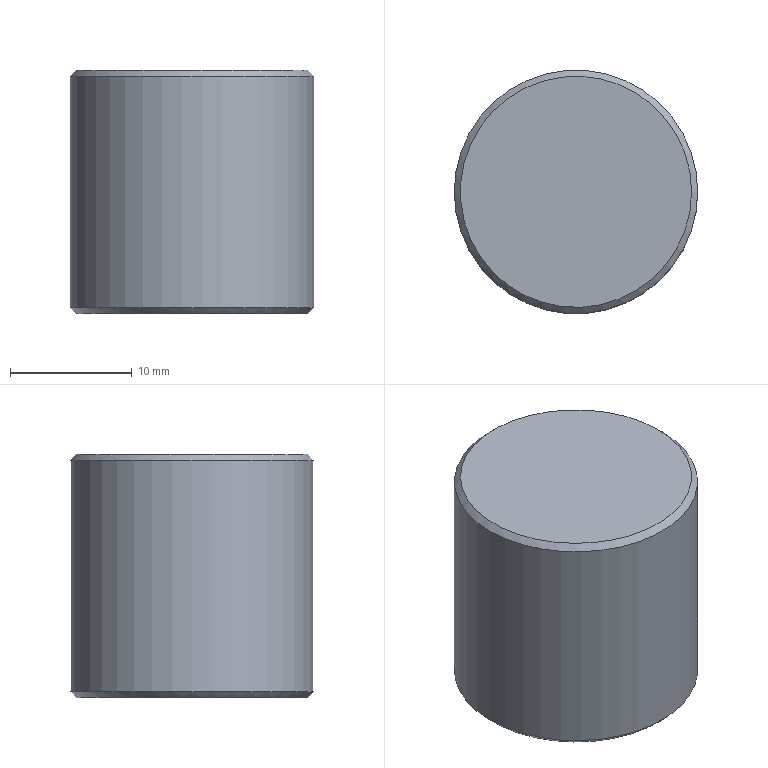Part | STEP file | E112002500 | 1 solid | 5 faces | box 20 x 20 x 20 mm | volume 6268 mm3 | plane 2 | cone 2 | cylinder 1 | commonest cylinder face diameters 20 x1
STEP:
#1=CARTESIAN_POINT('',(0.,0.,0.));
#2=DIRECTION('',(0.,0.,1.));
#3=DIRECTION('',(1.,0.,0.));
#4=AXIS2_PLACEMENT_3D('',#1,#2,#3);
#5=CARTESIAN_POINT('',(10.,0.,-0.5));
#6=VERTEX_POINT('',#5);
#7=CARTESIAN_POINT('',(0.,0.,-0.5));
#8=DIRECTION('',(0.,0.,-1.));
#9=DIRECTION('',(1.,0.,0.));
#10=AXIS2_PLACEMENT_3D('',#7,#8,#9);
#11=CIRCLE('',#10,10.);
#12=CARTESIAN_POINT('',(0.,0.,-20.));
#13=DIRECTION('',(0.,0.,1.));
#14=DIRECTION('',(1.,0.,0.));
#15=AXIS2_PLACEMENT_3D('',#12,#13,#14);
#16=CYLINDRICAL_SURFACE('',#15,10.);
#17=CARTESIAN_POINT('',(6.283,19.5));
#18=DIRECTION('',(-1.,0.));
#19=VECTOR('',#18,1.);
#20=LINE('',#17,#19);
#21=(GEOMETRIC_REPRESENTATION_CONTEXT(2)PARAMETRIC_REPRESENTATION_CONTEXT()REPRESENTATION_CONTEXT('',''));
#22=DEFINITIONAL_REPRESENTATION('',(#20),#21);
#23=PCURVE('',#16,#22);
#24=CARTESIAN_POINT('',(0.,0.,0.));
#25=DIRECTION('',(0.,0.,-1.));
#26=DIRECTION('',(-1.,0.,0.));
#27=AXIS2_PLACEMENT_3D('',#24,#25,#26);
#28=CONICAL_SURFACE('',#27,9.5,0.7854);
#29=CARTESIAN_POINT('',(3.142,0.5));
#30=DIRECTION('',(1.,0.));
#31=VECTOR('',#30,1.);
#32=LINE('',#29,#31);
#33=(GEOMETRIC_REPRESENTATION_CONTEXT(2)PARAMETRIC_REPRESENTATION_CONTEXT()REPRESENTATION_CONTEXT('',''));
#34=DEFINITIONAL_REPRESENTATION('',(#32),#33);
#35=PCURVE('',#28,#34);
#36=SURFACE_CURVE('',#11,(#23,#35),.PCURVE_S1.);
#37=EDGE_CURVE('',#6,#6,#36,.T.);
#38=ORIENTED_EDGE('',*,*,#37,.T.);
#39=CARTESIAN_POINT('',(10.,0.,-19.5));
#40=VERTEX_POINT('',#39);
#41=CARTESIAN_POINT('',(10.,0.,-19.5));
#42=CARTESIAN_POINT('',(10.,0.,-0.5));
#43=B_SPLINE_CURVE_WITH_KNOTS('',1,(#41,#42),.UNSPECIFIED.,.F.,.F.,(2,2),(0.5,19.5),.PIECEWISE_BEZIER_KNOTS.);
#44=CARTESIAN_POINT('',(0.,0.));
#45=DIRECTION('',(0.,1.));
#46=VECTOR('',#45,1.);
#47=LINE('',#44,#46);
#48=(GEOMETRIC_REPRESENTATION_CONTEXT(2)PARAMETRIC_REPRESENTATION_CONTEXT()REPRESENTATION_CONTEXT('',''));
#49=DEFINITIONAL_REPRESENTATION('',(#47),#48);
#50=PCURVE('',#16,#49);
#51=CARTESIAN_POINT('',(6.283,0.));
#52=DIRECTION('',(0.,1.));
#53=VECTOR('',#52,1.);
#54=LINE('',#51,#53);
#55=(GEOMETRIC_REPRESENTATION_CONTEXT(2)PARAMETRIC_REPRESENTATION_CONTEXT()REPRESENTATION_CONTEXT('',''));
#56=DEFINITIONAL_REPRESENTATION('',(#54),#55);
#57=PCURVE('',#16,#56);
#58=SEAM_CURVE('',#43,(#50,#57),.PCURVE_S1.);
#59=EDGE_CURVE('',#40,#6,#58,.T.);
#60=ORIENTED_EDGE('',*,*,#59,.F.);
#61=CARTESIAN_POINT('',(0.,0.,-19.5));
#62=DIRECTION('',(0.,0.,1.));
#63=DIRECTION('',(1.,0.,0.));
#64=AXIS2_PLACEMENT_3D('',#61,#62,#63);
#65=CIRCLE('',#64,10.);
#66=CARTESIAN_POINT('',(0.,0.5));
#67=DIRECTION('',(1.,0.));
#68=VECTOR('',#67,1.);
#69=LINE('',#66,#68);
#70=(GEOMETRIC_REPRESENTATION_CONTEXT(2)PARAMETRIC_REPRESENTATION_CONTEXT()REPRESENTATION_CONTEXT('',''));
#71=DEFINITIONAL_REPRESENTATION('',(#69),#70);
#72=PCURVE('',#16,#71);
#73=CARTESIAN_POINT('',(0.,0.,-19.5));
#74=DIRECTION('',(0.,0.,1.));
#75=DIRECTION('',(1.,0.,0.));
#76=AXIS2_PLACEMENT_3D('',#73,#74,#75);
#77=CONICAL_SURFACE('',#76,10.,0.7854);
#78=CARTESIAN_POINT('',(0.,0.));
#79=DIRECTION('',(1.,0.));
#80=VECTOR('',#79,1.);
#81=LINE('',#78,#80);
#82=(GEOMETRIC_REPRESENTATION_CONTEXT(2)PARAMETRIC_REPRESENTATION_CONTEXT()REPRESENTATION_CONTEXT('',''));
#83=DEFINITIONAL_REPRESENTATION('',(#81),#82);
#84=PCURVE('',#77,#83);
#85=SURFACE_CURVE('',#65,(#72,#84),.PCURVE_S1.);
#86=EDGE_CURVE('',#40,#40,#85,.T.);
#87=ORIENTED_EDGE('',*,*,#86,.T.);
#88=ORIENTED_EDGE('',*,*,#59,.T.);
#89=EDGE_LOOP('',(#38,#60,#87,#88));
#90=FACE_BOUND('',#89,.T.);
#91=ADVANCED_FACE('',(#90),#16,.T.);
#92=CARTESIAN_POINT('',(9.5,0.,-20.));
#93=VERTEX_POINT('',#92);
#94=CARTESIAN_POINT('',(0.,0.,-20.));
#95=DIRECTION('',(0.,0.,-1.));
#96=DIRECTION('',(1.,0.,0.));
#97=AXIS2_PLACEMENT_3D('',#94,#95,#96);
#98=CIRCLE('',#97,9.5);
#99=CARTESIAN_POINT('',(0.,0.,-20.));
#100=DIRECTION('',(0.,0.,1.));
#101=DIRECTION('',(1.,0.,0.));
#102=AXIS2_PLACEMENT_3D('',#99,#100,#101);
#103=PLANE('',#102);
#104=CARTESIAN_POINT('',(9.5,0.));
#105=CARTESIAN_POINT('',(9.5,-16.454));
#106=CARTESIAN_POINT('',(-4.75,-8.227));
#107=CARTESIAN_POINT('',(-19.,0.));
#108=CARTESIAN_POINT('',(-4.75,8.227));
#109=CARTESIAN_POINT('',(9.5,16.454));
#110=CARTESIAN_POINT('',(9.5,0.));
#111=(BOUNDED_CURVE()B_SPLINE_CURVE(2,(#104,#105,#106,#107,#108,#109,#110),.UNSPECIFIED.,.T.,.F.)B_SPLINE_CURVE_WITH_KNOTS((1,2,2,2,2,1),(-2.094,0.,2.094,4.189,6.283,8.378),.UNSPECIFIED.)CURVE()GEOMETRIC_REPRESENTATION_ITEM()RATIONAL_B_SPLINE_CURVE((1.,0.5,1.,0.5,1.,0.5,1.))REPRESENTATION_ITEM(''));
#112=(GEOMETRIC_REPRESENTATION_CONTEXT(2)PARAMETRIC_REPRESENTATION_CONTEXT()REPRESENTATION_CONTEXT('',''));
#113=DEFINITIONAL_REPRESENTATION('',(#111),#112);
#114=PCURVE('',#103,#113);
#115=CARTESIAN_POINT('',(6.283,-0.5));
#116=DIRECTION('',(-1.,0.));
#117=VECTOR('',#116,1.);
#118=LINE('',#115,#117);
#119=(GEOMETRIC_REPRESENTATION_CONTEXT(2)PARAMETRIC_REPRESENTATION_CONTEXT()REPRESENTATION_CONTEXT('',''));
#120=DEFINITIONAL_REPRESENTATION('',(#118),#119);
#121=PCURVE('',#77,#120);
#122=SURFACE_CURVE('',#98,(#114,#121),.PCURVE_S1.);
#123=EDGE_CURVE('',#93,#93,#122,.T.);
#124=ORIENTED_EDGE('',*,*,#123,.T.);
#125=EDGE_LOOP('',(#124));
#126=FACE_BOUND('',#125,.T.);
#127=ADVANCED_FACE('',(#126),#103,.F.);
#128=CARTESIAN_POINT('',(9.5,0.,0.));
#129=VERTEX_POINT('',#128);
#130=CARTESIAN_POINT('',(0.,0.,0.));
#131=DIRECTION('',(0.,0.,1.));
#132=DIRECTION('',(1.,0.,0.));
#133=AXIS2_PLACEMENT_3D('',#130,#131,#132);
#134=CIRCLE('',#133,9.5);
#135=CARTESIAN_POINT('',(0.,0.,0.));
#136=DIRECTION('',(0.,0.,1.));
#137=DIRECTION('',(1.,0.,0.));
#138=AXIS2_PLACEMENT_3D('',#135,#136,#137);
#139=PLANE('',#138);
#140=CARTESIAN_POINT('',(0.,0.));
#141=DIRECTION('',(1.,0.));
#142=AXIS2_PLACEMENT_2D('',#140,#141);
#143=CIRCLE('',#142,9.5);
#144=(GEOMETRIC_REPRESENTATION_CONTEXT(2)PARAMETRIC_REPRESENTATION_CONTEXT()REPRESENTATION_CONTEXT('',''));
#145=DEFINITIONAL_REPRESENTATION('',(#143),#144);
#146=PCURVE('',#139,#145);
#147=CARTESIAN_POINT('',(9.425,0.));
#148=DIRECTION('',(-1.,0.));
#149=VECTOR('',#148,1.);
#150=LINE('',#147,#149);
#151=(GEOMETRIC_REPRESENTATION_CONTEXT(2)PARAMETRIC_REPRESENTATION_CONTEXT()REPRESENTATION_CONTEXT('',''));
#152=DEFINITIONAL_REPRESENTATION('',(#150),#151);
#153=PCURVE('',#28,#152);
#154=SURFACE_CURVE('',#134,(#146,#153),.PCURVE_S1.);
#155=EDGE_CURVE('',#129,#129,#154,.T.);
#156=ORIENTED_EDGE('',*,*,#155,.T.);
#157=EDGE_LOOP('',(#156));
#158=FACE_BOUND('',#157,.T.);
#159=ADVANCED_FACE('',(#158),#139,.T.);
#160=ORIENTED_EDGE('',*,*,#37,.F.);
#161=CARTESIAN_POINT('',(9.5,0.,0.));
#162=CARTESIAN_POINT('',(10.,0.,-0.5));
#163=B_SPLINE_CURVE_WITH_KNOTS('',1,(#161,#162),.UNSPECIFIED.,.F.,.F.,(2,2),(0.,0.7071),.PIECEWISE_BEZIER_KNOTS.);
#164=CARTESIAN_POINT('',(3.142,0.));
#165=DIRECTION('',(0.,1.));
#166=VECTOR('',#165,1.);
#167=LINE('',#164,#166);
#168=(GEOMETRIC_REPRESENTATION_CONTEXT(2)PARAMETRIC_REPRESENTATION_CONTEXT()REPRESENTATION_CONTEXT('',''));
#169=DEFINITIONAL_REPRESENTATION('',(#167),#168);
#170=PCURVE('',#28,#169);
#171=CARTESIAN_POINT('',(9.425,0.));
#172=DIRECTION('',(0.,1.));
#173=VECTOR('',#172,1.);
#174=LINE('',#171,#173);
#175=(GEOMETRIC_REPRESENTATION_CONTEXT(2)PARAMETRIC_REPRESENTATION_CONTEXT()REPRESENTATION_CONTEXT('',''));
#176=DEFINITIONAL_REPRESENTATION('',(#174),#175);
#177=PCURVE('',#28,#176);
#178=SEAM_CURVE('',#163,(#170,#177),.PCURVE_S1.);
#179=EDGE_CURVE('',#129,#6,#178,.T.);
#180=ORIENTED_EDGE('',*,*,#179,.F.);
#181=ORIENTED_EDGE('',*,*,#155,.F.);
#182=ORIENTED_EDGE('',*,*,#179,.T.);
#183=EDGE_LOOP('',(#160,#180,#181,#182));
#184=FACE_BOUND('',#183,.T.);
#185=ADVANCED_FACE('',(#184),#28,.T.);
#186=ORIENTED_EDGE('',*,*,#123,.F.);
#187=CARTESIAN_POINT('',(9.5,0.,-20.));
#188=CARTESIAN_POINT('',(10.,0.,-19.5));
#189=B_SPLINE_CURVE_WITH_KNOTS('',1,(#187,#188),.UNSPECIFIED.,.F.,.F.,(2,2),(-0.7071,0.),.PIECEWISE_BEZIER_KNOTS.);
#190=CARTESIAN_POINT('',(6.283,0.));
#191=DIRECTION('',(0.,1.));
#192=VECTOR('',#191,1.);
#193=LINE('',#190,#192);
#194=(GEOMETRIC_REPRESENTATION_CONTEXT(2)PARAMETRIC_REPRESENTATION_CONTEXT()REPRESENTATION_CONTEXT('',''));
#195=DEFINITIONAL_REPRESENTATION('',(#193),#194);
#196=PCURVE('',#77,#195);
#197=CARTESIAN_POINT('',(0.,0.));
#198=DIRECTION('',(0.,1.));
#199=VECTOR('',#198,1.);
#200=LINE('',#197,#199);
#201=(GEOMETRIC_REPRESENTATION_CONTEXT(2)PARAMETRIC_REPRESENTATION_CONTEXT()REPRESENTATION_CONTEXT('',''));
#202=DEFINITIONAL_REPRESENTATION('',(#200),#201);
#203=PCURVE('',#77,#202);
#204=SEAM_CURVE('',#189,(#196,#203),.PCURVE_S1.);
#205=EDGE_CURVE('',#93,#40,#204,.T.);
#206=ORIENTED_EDGE('',*,*,#205,.T.);
#207=ORIENTED_EDGE('',*,*,#86,.F.);
#208=ORIENTED_EDGE('',*,*,#205,.F.);
#209=EDGE_LOOP('',(#186,#206,#207,#208));
#210=FACE_BOUND('',#209,.T.);
#211=ADVANCED_FACE('',(#210),#77,.T.);
#212=CLOSED_SHELL('',(#91,#127,#159,#185,#211));
#213=MANIFOLD_SOLID_BREP('',#212);
#214=(LENGTH_UNIT()NAMED_UNIT(*)SI_UNIT(.MILLI.,.METRE.));
#215=UNCERTAINTY_MEASURE_WITH_UNIT(LENGTH_MEASURE(0.00001),#214,'','');
#216=(NAMED_UNIT(*)PLANE_ANGLE_UNIT()SI_UNIT($,.RADIAN.));
#217=(NAMED_UNIT(*)SI_UNIT($,.STERADIAN.)SOLID_ANGLE_UNIT());
#218=(GEOMETRIC_REPRESENTATION_CONTEXT(3)GLOBAL_UNCERTAINTY_ASSIGNED_CONTEXT((#215))GLOBAL_UNIT_ASSIGNED_CONTEXT((#214,#216,#217))REPRESENTATION_CONTEXT('',''));
#219=ADVANCED_BREP_SHAPE_REPRESENTATION('',(#4,#213),#218);